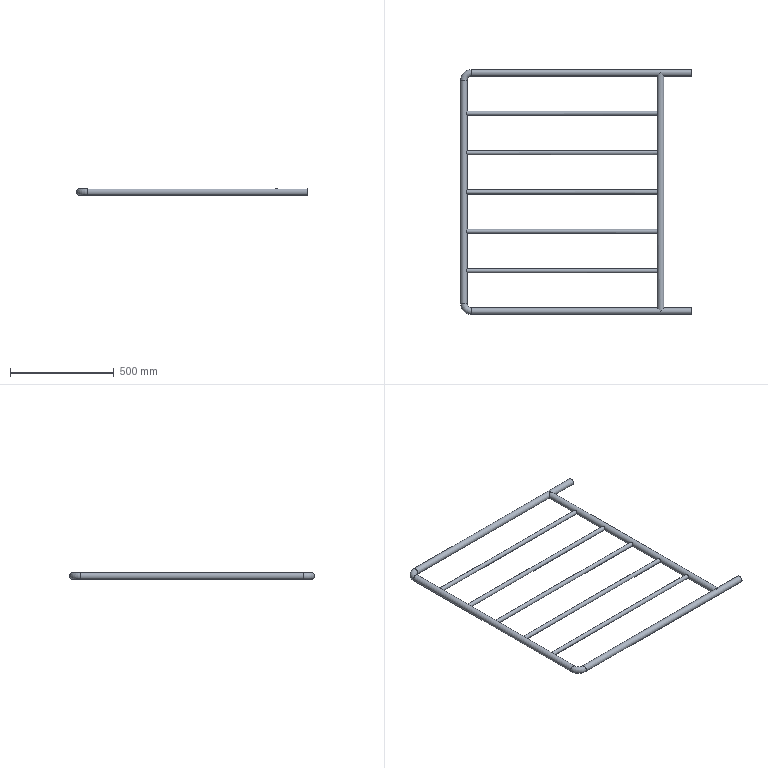Part | STEP file | 304 guardrail 1150X1100 body_Default<As Machined> | 11 solids | 44 faces | box 1116 x 1182 x 32 mm | volume 913541 mm3 | cylinder 30 | plane 10 | torus 4 | commonest cylinder face diameters 32 x16 18 x5 20 x5 29 x4